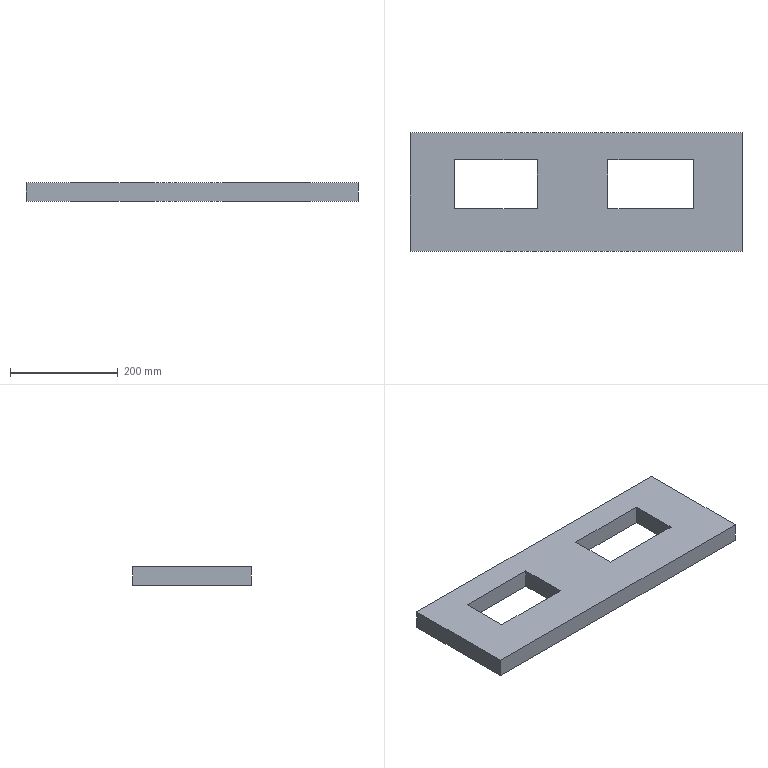Part | SolidWorks | features Extrusion 1, ICE 1 | 1 solid | 14 faces | box 616 x 220 x 35 mm | volume 3748166 mm3 | plane 14
STEP:
#1=CARTESIAN_POINT('',(308.,0.,17.5));
#2=VERTEX_POINT('',#1);
#3=CARTESIAN_POINT('',(308.,0.,-17.5));
#4=VERTEX_POINT('',#3);
#5=CARTESIAN_POINT('',(308.,0.,17.5));
#6=DIRECTION('',(0.,0.,-1.));
#7=VECTOR('',#6,1000.);
#8=LINE('',#5,#7);
#9=EDGE_CURVE('',#2,#4,#8,.T.);
#10=ORIENTED_EDGE('',*,*,#9,.T.);
#11=CARTESIAN_POINT('',(308.,220.,-17.5));
#12=VERTEX_POINT('',#11);
#13=CARTESIAN_POINT('',(308.,220.,-17.5));
#14=DIRECTION('',(0.,-1.,0.));
#15=VECTOR('',#14,1000.);
#16=LINE('',#13,#15);
#17=EDGE_CURVE('',#12,#4,#16,.T.);
#18=ORIENTED_EDGE('',*,*,#17,.F.);
#19=CARTESIAN_POINT('',(308.,220.,17.5));
#20=VERTEX_POINT('',#19);
#21=CARTESIAN_POINT('',(308.,220.,17.5));
#22=DIRECTION('',(0.,0.,-1.));
#23=VECTOR('',#22,1000.);
#24=LINE('',#21,#23);
#25=EDGE_CURVE('',#20,#12,#24,.T.);
#26=ORIENTED_EDGE('',*,*,#25,.F.);
#27=CARTESIAN_POINT('',(308.,220.,17.5));
#28=DIRECTION('',(0.,-1.,0.));
#29=VECTOR('',#28,1000.);
#30=LINE('',#27,#29);
#31=EDGE_CURVE('',#20,#2,#30,.T.);
#32=ORIENTED_EDGE('',*,*,#31,.T.);
#33=EDGE_LOOP('',(#10,#18,#26,#32));
#34=FACE_OUTER_BOUND('',#33,.T.);
#35=CARTESIAN_POINT('',(308.,220.,17.5));
#36=DIRECTION('',(-1.,0.,0.));
#37=DIRECTION('',(0.,0.,1.));
#38=AXIS2_PLACEMENT_3D('',#35,#36,#37);
#39=PLANE('',#38);
#40=ADVANCED_FACE('',(#34),#39,.F.);
#41=CARTESIAN_POINT('',(-225.575,79.078,-17.5));
#42=VERTEX_POINT('',#41);
#43=CARTESIAN_POINT('',(-71.632,79.078,-17.5));
#44=VERTEX_POINT('',#43);
#45=CARTESIAN_POINT('',(-225.575,79.078,-17.5));
#46=DIRECTION('',(1.,0.,0.));
#47=VECTOR('',#46,1000.);
#48=LINE('',#45,#47);
#49=EDGE_CURVE('',#42,#44,#48,.T.);
#50=ORIENTED_EDGE('',*,*,#49,.T.);
#51=CARTESIAN_POINT('',(-71.632,169.842,-17.5));
#52=VERTEX_POINT('',#51);
#53=CARTESIAN_POINT('',(-71.632,169.842,-17.5));
#54=DIRECTION('',(0.,1.,0.));
#55=VECTOR('',#54,1000.);
#56=LINE('',#53,#55);
#57=EDGE_CURVE('',#44,#52,#56,.T.);
#58=ORIENTED_EDGE('',*,*,#57,.T.);
#59=CARTESIAN_POINT('',(-225.575,169.842,-17.5));
#60=VERTEX_POINT('',#59);
#61=CARTESIAN_POINT('',(-225.575,169.842,-17.5));
#62=DIRECTION('',(-1.,0.,0.));
#63=VECTOR('',#62,1000.);
#64=LINE('',#61,#63);
#65=EDGE_CURVE('',#52,#60,#64,.T.);
#66=ORIENTED_EDGE('',*,*,#65,.T.);
#67=CARTESIAN_POINT('',(-225.575,169.842,-17.5));
#68=DIRECTION('',(0.,-1.,0.));
#69=VECTOR('',#68,1000.);
#70=LINE('',#67,#69);
#71=EDGE_CURVE('',#60,#42,#70,.T.);
#72=ORIENTED_EDGE('',*,*,#71,.T.);
#73=EDGE_LOOP('',(#50,#58,#66,#72));
#74=FACE_BOUND('',#73,.T.);
#75=CARTESIAN_POINT('',(59.175,79.078,-17.5));
#76=VERTEX_POINT('',#75);
#77=CARTESIAN_POINT('',(218.456,79.078,-17.5));
#78=VERTEX_POINT('',#77);
#79=CARTESIAN_POINT('',(59.175,79.078,-17.5));
#80=DIRECTION('',(1.,0.,0.));
#81=VECTOR('',#80,1000.);
#82=LINE('',#79,#81);
#83=EDGE_CURVE('',#76,#78,#82,.T.);
#84=ORIENTED_EDGE('',*,*,#83,.T.);
#85=CARTESIAN_POINT('',(218.456,169.842,-17.5));
#86=VERTEX_POINT('',#85);
#87=CARTESIAN_POINT('',(218.456,79.078,-17.5));
#88=DIRECTION('',(0.,1.,0.));
#89=VECTOR('',#88,1000.);
#90=LINE('',#87,#89);
#91=EDGE_CURVE('',#78,#86,#90,.T.);
#92=ORIENTED_EDGE('',*,*,#91,.T.);
#93=CARTESIAN_POINT('',(59.175,169.842,-17.5));
#94=VERTEX_POINT('',#93);
#95=CARTESIAN_POINT('',(59.175,169.842,-17.5));
#96=DIRECTION('',(-1.,0.,0.));
#97=VECTOR('',#96,1000.);
#98=LINE('',#95,#97);
#99=EDGE_CURVE('',#86,#94,#98,.T.);
#100=ORIENTED_EDGE('',*,*,#99,.T.);
#101=CARTESIAN_POINT('',(59.175,79.078,-17.5));
#102=DIRECTION('',(0.,-1.,0.));
#103=VECTOR('',#102,1000.);
#104=LINE('',#101,#103);
#105=EDGE_CURVE('',#94,#76,#104,.T.);
#106=ORIENTED_EDGE('',*,*,#105,.T.);
#107=EDGE_LOOP('',(#84,#92,#100,#106));
#108=FACE_BOUND('',#107,.T.);
#109=CARTESIAN_POINT('',(-308.,0.,-17.5));
#110=VERTEX_POINT('',#109);
#111=CARTESIAN_POINT('',(-308.,0.,-17.5));
#112=DIRECTION('',(-1.,0.,0.));
#113=VECTOR('',#112,1000.);
#114=LINE('',#111,#113);
#115=EDGE_CURVE('',#4,#110,#114,.T.);
#116=ORIENTED_EDGE('',*,*,#115,.T.);
#117=CARTESIAN_POINT('',(-308.,220.,-17.5));
#118=VERTEX_POINT('',#117);
#119=CARTESIAN_POINT('',(-308.,220.,-17.5));
#120=DIRECTION('',(0.,-1.,0.));
#121=VECTOR('',#120,1000.);
#122=LINE('',#119,#121);
#123=EDGE_CURVE('',#118,#110,#122,.T.);
#124=ORIENTED_EDGE('',*,*,#123,.F.);
#125=CARTESIAN_POINT('',(-308.,220.,-17.5));
#126=DIRECTION('',(-1.,0.,0.));
#127=VECTOR('',#126,1000.);
#128=LINE('',#125,#127);
#129=EDGE_CURVE('',#12,#118,#128,.T.);
#130=ORIENTED_EDGE('',*,*,#129,.F.);
#131=ORIENTED_EDGE('',*,*,#17,.T.);
#132=EDGE_LOOP('',(#116,#124,#130,#131));
#133=FACE_OUTER_BOUND('',#132,.T.);
#134=CARTESIAN_POINT('',(-308.,220.,-17.5));
#135=DIRECTION('',(0.,0.,1.));
#136=DIRECTION('',(1.,0.,0.));
#137=AXIS2_PLACEMENT_3D('',#134,#135,#136);
#138=PLANE('',#137);
#139=ADVANCED_FACE('',(#74,#108,#133),#138,.F.);
#140=CARTESIAN_POINT('',(-308.,0.,17.5));
#141=VERTEX_POINT('',#140);
#142=CARTESIAN_POINT('',(-308.,0.,17.5));
#143=DIRECTION('',(0.,0.,1.));
#144=VECTOR('',#143,1000.);
#145=LINE('',#142,#144);
#146=EDGE_CURVE('',#110,#141,#145,.T.);
#147=ORIENTED_EDGE('',*,*,#146,.T.);
#148=CARTESIAN_POINT('',(-308.,220.,17.5));
#149=VERTEX_POINT('',#148);
#150=CARTESIAN_POINT('',(-308.,220.,17.5));
#151=DIRECTION('',(0.,-1.,0.));
#152=VECTOR('',#151,1000.);
#153=LINE('',#150,#152);
#154=EDGE_CURVE('',#149,#141,#153,.T.);
#155=ORIENTED_EDGE('',*,*,#154,.F.);
#156=CARTESIAN_POINT('',(-308.,220.,17.5));
#157=DIRECTION('',(0.,0.,1.));
#158=VECTOR('',#157,1000.);
#159=LINE('',#156,#158);
#160=EDGE_CURVE('',#118,#149,#159,.T.);
#161=ORIENTED_EDGE('',*,*,#160,.F.);
#162=ORIENTED_EDGE('',*,*,#123,.T.);
#163=EDGE_LOOP('',(#147,#155,#161,#162));
#164=FACE_OUTER_BOUND('',#163,.T.);
#165=CARTESIAN_POINT('',(-308.,220.,17.5));
#166=DIRECTION('',(1.,0.,0.));
#167=DIRECTION('',(0.,0.,-1.));
#168=AXIS2_PLACEMENT_3D('',#165,#166,#167);
#169=PLANE('',#168);
#170=ADVANCED_FACE('',(#164),#169,.F.);
#171=CARTESIAN_POINT('',(-71.632,169.842,17.5));
#172=VERTEX_POINT('',#171);
#173=CARTESIAN_POINT('',(-225.575,169.842,17.5));
#174=VERTEX_POINT('',#173);
#175=CARTESIAN_POINT('',(-225.575,169.842,17.5));
#176=DIRECTION('',(-1.,0.,0.));
#177=VECTOR('',#176,1000.);
#178=LINE('',#175,#177);
#179=EDGE_CURVE('',#172,#174,#178,.T.);
#180=ORIENTED_EDGE('',*,*,#179,.F.);
#181=CARTESIAN_POINT('',(-71.632,79.078,17.5));
#182=VERTEX_POINT('',#181);
#183=CARTESIAN_POINT('',(-71.632,169.842,17.5));
#184=DIRECTION('',(0.,1.,0.));
#185=VECTOR('',#184,1000.);
#186=LINE('',#183,#185);
#187=EDGE_CURVE('',#182,#172,#186,.T.);
#188=ORIENTED_EDGE('',*,*,#187,.F.);
#189=CARTESIAN_POINT('',(-225.575,79.078,17.5));
#190=VERTEX_POINT('',#189);
#191=CARTESIAN_POINT('',(-225.575,79.078,17.5));
#192=DIRECTION('',(1.,0.,0.));
#193=VECTOR('',#192,1000.);
#194=LINE('',#191,#193);
#195=EDGE_CURVE('',#190,#182,#194,.T.);
#196=ORIENTED_EDGE('',*,*,#195,.F.);
#197=CARTESIAN_POINT('',(-225.575,169.842,17.5));
#198=DIRECTION('',(0.,-1.,0.));
#199=VECTOR('',#198,1000.);
#200=LINE('',#197,#199);
#201=EDGE_CURVE('',#174,#190,#200,.T.);
#202=ORIENTED_EDGE('',*,*,#201,.F.);
#203=EDGE_LOOP('',(#180,#188,#196,#202));
#204=FACE_BOUND('',#203,.T.);
#205=CARTESIAN_POINT('',(218.456,169.842,17.5));
#206=VERTEX_POINT('',#205);
#207=CARTESIAN_POINT('',(59.175,169.842,17.5));
#208=VERTEX_POINT('',#207);
#209=CARTESIAN_POINT('',(59.175,169.842,17.5));
#210=DIRECTION('',(-1.,0.,0.));
#211=VECTOR('',#210,1000.);
#212=LINE('',#209,#211);
#213=EDGE_CURVE('',#206,#208,#212,.T.);
#214=ORIENTED_EDGE('',*,*,#213,.F.);
#215=CARTESIAN_POINT('',(218.456,79.078,17.5));
#216=VERTEX_POINT('',#215);
#217=CARTESIAN_POINT('',(218.456,79.078,17.5));
#218=DIRECTION('',(0.,1.,0.));
#219=VECTOR('',#218,1000.);
#220=LINE('',#217,#219);
#221=EDGE_CURVE('',#216,#206,#220,.T.);
#222=ORIENTED_EDGE('',*,*,#221,.F.);
#223=CARTESIAN_POINT('',(59.175,79.078,17.5));
#224=VERTEX_POINT('',#223);
#225=CARTESIAN_POINT('',(59.175,79.078,17.5));
#226=DIRECTION('',(1.,0.,0.));
#227=VECTOR('',#226,1000.);
#228=LINE('',#225,#227);
#229=EDGE_CURVE('',#224,#216,#228,.T.);
#230=ORIENTED_EDGE('',*,*,#229,.F.);
#231=CARTESIAN_POINT('',(59.175,79.078,17.5));
#232=DIRECTION('',(0.,-1.,0.));
#233=VECTOR('',#232,1000.);
#234=LINE('',#231,#233);
#235=EDGE_CURVE('',#208,#224,#234,.T.);
#236=ORIENTED_EDGE('',*,*,#235,.F.);
#237=EDGE_LOOP('',(#214,#222,#230,#236));
#238=FACE_BOUND('',#237,.T.);
#239=CARTESIAN_POINT('',(-308.,0.,17.5));
#240=DIRECTION('',(1.,0.,0.));
#241=VECTOR('',#240,1000.);
#242=LINE('',#239,#241);
#243=EDGE_CURVE('',#141,#2,#242,.T.);
#244=ORIENTED_EDGE('',*,*,#243,.T.);
#245=ORIENTED_EDGE('',*,*,#31,.F.);
#246=CARTESIAN_POINT('',(-308.,220.,17.5));
#247=DIRECTION('',(1.,0.,0.));
#248=VECTOR('',#247,1000.);
#249=LINE('',#246,#248);
#250=EDGE_CURVE('',#149,#20,#249,.T.);
#251=ORIENTED_EDGE('',*,*,#250,.F.);
#252=ORIENTED_EDGE('',*,*,#154,.T.);
#253=EDGE_LOOP('',(#244,#245,#251,#252));
#254=FACE_OUTER_BOUND('',#253,.T.);
#255=CARTESIAN_POINT('',(-308.,220.,17.5));
#256=DIRECTION('',(0.,0.,-1.));
#257=DIRECTION('',(-1.,0.,0.));
#258=AXIS2_PLACEMENT_3D('',#255,#256,#257);
#259=PLANE('',#258);
#260=ADVANCED_FACE('',(#204,#238,#254),#259,.F.);
#261=ORIENTED_EDGE('',*,*,#25,.T.);
#262=ORIENTED_EDGE('',*,*,#129,.T.);
#263=ORIENTED_EDGE('',*,*,#160,.T.);
#264=ORIENTED_EDGE('',*,*,#250,.T.);
#265=EDGE_LOOP('',(#261,#262,#263,#264));
#266=FACE_OUTER_BOUND('',#265,.T.);
#267=CARTESIAN_POINT('',(0.,220.,0.));
#268=DIRECTION('',(0.,-1.,0.));
#269=DIRECTION('',(0.,0.,-1.));
#270=AXIS2_PLACEMENT_3D('',#267,#268,#269);
#271=PLANE('',#270);
#272=ADVANCED_FACE('',(#266),#271,.F.);
#273=ORIENTED_EDGE('',*,*,#9,.F.);
#274=ORIENTED_EDGE('',*,*,#243,.F.);
#275=ORIENTED_EDGE('',*,*,#146,.F.);
#276=ORIENTED_EDGE('',*,*,#115,.F.);
#277=EDGE_LOOP('',(#273,#274,#275,#276));
#278=FACE_OUTER_BOUND('',#277,.T.);
#279=CARTESIAN_POINT('',(0.,0.,0.));
#280=DIRECTION('',(0.,-1.,0.));
#281=DIRECTION('',(0.,0.,-1.));
#282=AXIS2_PLACEMENT_3D('',#279,#280,#281);
#283=PLANE('',#282);
#284=ADVANCED_FACE('',(#278),#283,.T.);
#285=ORIENTED_EDGE('',*,*,#221,.T.);
#286=CARTESIAN_POINT('',(218.456,169.842,-17.5));
#287=DIRECTION('',(0.,0.,1.));
#288=VECTOR('',#287,1000.);
#289=LINE('',#286,#288);
#290=EDGE_CURVE('',#86,#206,#289,.T.);
#291=ORIENTED_EDGE('',*,*,#290,.F.);
#292=ORIENTED_EDGE('',*,*,#91,.F.);
#293=CARTESIAN_POINT('',(218.456,79.078,-17.5));
#294=DIRECTION('',(0.,0.,1.));
#295=VECTOR('',#294,1000.);
#296=LINE('',#293,#295);
#297=EDGE_CURVE('',#78,#216,#296,.T.);
#298=ORIENTED_EDGE('',*,*,#297,.T.);
#299=EDGE_LOOP('',(#285,#291,#292,#298));
#300=FACE_OUTER_BOUND('',#299,.T.);
#301=CARTESIAN_POINT('',(218.456,79.078,-17.5));
#302=DIRECTION('',(1.,0.,0.));
#303=DIRECTION('',(0.,0.,-1.));
#304=AXIS2_PLACEMENT_3D('',#301,#302,#303);
#305=PLANE('',#304);
#306=ADVANCED_FACE('',(#300),#305,.F.);
#307=ORIENTED_EDGE('',*,*,#229,.T.);
#308=ORIENTED_EDGE('',*,*,#297,.F.);
#309=ORIENTED_EDGE('',*,*,#83,.F.);
#310=CARTESIAN_POINT('',(59.175,79.078,-17.5));
#311=DIRECTION('',(0.,0.,1.));
#312=VECTOR('',#311,1000.);
#313=LINE('',#310,#312);
#314=EDGE_CURVE('',#76,#224,#313,.T.);
#315=ORIENTED_EDGE('',*,*,#314,.T.);
#316=EDGE_LOOP('',(#307,#308,#309,#315));
#317=FACE_OUTER_BOUND('',#316,.T.);
#318=CARTESIAN_POINT('',(59.175,79.078,-17.5));
#319=DIRECTION('',(0.,-1.,0.));
#320=DIRECTION('',(0.,0.,-1.));
#321=AXIS2_PLACEMENT_3D('',#318,#319,#320);
#322=PLANE('',#321);
#323=ADVANCED_FACE('',(#317),#322,.F.);
#324=ORIENTED_EDGE('',*,*,#235,.T.);
#325=ORIENTED_EDGE('',*,*,#314,.F.);
#326=ORIENTED_EDGE('',*,*,#105,.F.);
#327=CARTESIAN_POINT('',(59.175,169.842,-17.5));
#328=DIRECTION('',(0.,0.,1.));
#329=VECTOR('',#328,1000.);
#330=LINE('',#327,#329);
#331=EDGE_CURVE('',#94,#208,#330,.T.);
#332=ORIENTED_EDGE('',*,*,#331,.T.);
#333=EDGE_LOOP('',(#324,#325,#326,#332));
#334=FACE_OUTER_BOUND('',#333,.T.);
#335=CARTESIAN_POINT('',(59.175,79.078,-17.5));
#336=DIRECTION('',(-1.,0.,0.));
#337=DIRECTION('',(0.,0.,1.));
#338=AXIS2_PLACEMENT_3D('',#335,#336,#337);
#339=PLANE('',#338);
#340=ADVANCED_FACE('',(#334),#339,.F.);
#341=ORIENTED_EDGE('',*,*,#213,.T.);
#342=ORIENTED_EDGE('',*,*,#331,.F.);
#343=ORIENTED_EDGE('',*,*,#99,.F.);
#344=ORIENTED_EDGE('',*,*,#290,.T.);
#345=EDGE_LOOP('',(#341,#342,#343,#344));
#346=FACE_OUTER_BOUND('',#345,.T.);
#347=CARTESIAN_POINT('',(59.175,169.842,-17.5));
#348=DIRECTION('',(0.,1.,0.));
#349=DIRECTION('',(0.,0.,1.));
#350=AXIS2_PLACEMENT_3D('',#347,#348,#349);
#351=PLANE('',#350);
#352=ADVANCED_FACE('',(#346),#351,.F.);
#353=ORIENTED_EDGE('',*,*,#187,.T.);
#354=CARTESIAN_POINT('',(-71.632,169.842,-17.5));
#355=DIRECTION('',(0.,0.,1.));
#356=VECTOR('',#355,1000.);
#357=LINE('',#354,#356);
#358=EDGE_CURVE('',#52,#172,#357,.T.);
#359=ORIENTED_EDGE('',*,*,#358,.F.);
#360=ORIENTED_EDGE('',*,*,#57,.F.);
#361=CARTESIAN_POINT('',(-71.632,79.078,-17.5));
#362=DIRECTION('',(0.,0.,1.));
#363=VECTOR('',#362,1000.);
#364=LINE('',#361,#363);
#365=EDGE_CURVE('',#44,#182,#364,.T.);
#366=ORIENTED_EDGE('',*,*,#365,.T.);
#367=EDGE_LOOP('',(#353,#359,#360,#366));
#368=FACE_OUTER_BOUND('',#367,.T.);
#369=CARTESIAN_POINT('',(-71.632,169.842,-17.5));
#370=DIRECTION('',(1.,0.,0.));
#371=DIRECTION('',(0.,0.,-1.));
#372=AXIS2_PLACEMENT_3D('',#369,#370,#371);
#373=PLANE('',#372);
#374=ADVANCED_FACE('',(#368),#373,.F.);
#375=ORIENTED_EDGE('',*,*,#195,.T.);
#376=ORIENTED_EDGE('',*,*,#365,.F.);
#377=ORIENTED_EDGE('',*,*,#49,.F.);
#378=CARTESIAN_POINT('',(-225.575,79.078,-17.5));
#379=DIRECTION('',(0.,0.,1.));
#380=VECTOR('',#379,1000.);
#381=LINE('',#378,#380);
#382=EDGE_CURVE('',#42,#190,#381,.T.);
#383=ORIENTED_EDGE('',*,*,#382,.T.);
#384=EDGE_LOOP('',(#375,#376,#377,#383));
#385=FACE_OUTER_BOUND('',#384,.T.);
#386=CARTESIAN_POINT('',(-225.575,79.078,-17.5));
#387=DIRECTION('',(0.,-1.,0.));
#388=DIRECTION('',(0.,0.,-1.));
#389=AXIS2_PLACEMENT_3D('',#386,#387,#388);
#390=PLANE('',#389);
#391=ADVANCED_FACE('',(#385),#390,.F.);
#392=ORIENTED_EDGE('',*,*,#201,.T.);
#393=ORIENTED_EDGE('',*,*,#382,.F.);
#394=ORIENTED_EDGE('',*,*,#71,.F.);
#395=CARTESIAN_POINT('',(-225.575,169.842,-17.5));
#396=DIRECTION('',(0.,0.,1.));
#397=VECTOR('',#396,1000.);
#398=LINE('',#395,#397);
#399=EDGE_CURVE('',#60,#174,#398,.T.);
#400=ORIENTED_EDGE('',*,*,#399,.T.);
#401=EDGE_LOOP('',(#392,#393,#394,#400));
#402=FACE_OUTER_BOUND('',#401,.T.);
#403=CARTESIAN_POINT('',(-225.575,169.842,-17.5));
#404=DIRECTION('',(-1.,0.,0.));
#405=DIRECTION('',(0.,0.,1.));
#406=AXIS2_PLACEMENT_3D('',#403,#404,#405);
#407=PLANE('',#406);
#408=ADVANCED_FACE('',(#402),#407,.F.);
#409=ORIENTED_EDGE('',*,*,#179,.T.);
#410=ORIENTED_EDGE('',*,*,#399,.F.);
#411=ORIENTED_EDGE('',*,*,#65,.F.);
#412=ORIENTED_EDGE('',*,*,#358,.T.);
#413=EDGE_LOOP('',(#409,#410,#411,#412));
#414=FACE_OUTER_BOUND('',#413,.T.);
#415=CARTESIAN_POINT('',(-225.575,169.842,-17.5));
#416=DIRECTION('',(0.,1.,0.));
#417=DIRECTION('',(0.,0.,1.));
#418=AXIS2_PLACEMENT_3D('',#415,#416,#417);
#419=PLANE('',#418);
#420=ADVANCED_FACE('',(#414),#419,.F.);
#421=CLOSED_SHELL('',(#40,#139,#170,#260,#272,#284,#306,#323,#340,#352,#374,#391,#408,#420));
#422=MANIFOLD_SOLID_BREP('',#421);
#423=CARTESIAN_POINT('',(0.,0.,0.));
#424=DIRECTION('',(0.,0.,1.));
#425=DIRECTION('',(1.,0.,0.));
#426=AXIS2_PLACEMENT_3D('',#423,#424,#425);
#427=(LENGTH_UNIT()NAMED_UNIT(*)SI_UNIT(.MILLI.,.METRE.));
#428=UNCERTAINTY_MEASURE_WITH_UNIT(LENGTH_MEASURE(0.00001),#427,'','');
#429=(NAMED_UNIT(*)PLANE_ANGLE_UNIT()SI_UNIT($,.RADIAN.));
#430=(NAMED_UNIT(*)SI_UNIT($,.STERADIAN.)SOLID_ANGLE_UNIT());
#431=(GEOMETRIC_REPRESENTATION_CONTEXT(3)GLOBAL_UNCERTAINTY_ASSIGNED_CONTEXT((#428))GLOBAL_UNIT_ASSIGNED_CONTEXT((#427,#429,#430))REPRESENTATION_CONTEXT('',''));
#432=ADVANCED_BREP_SHAPE_REPRESENTATION('',(#422,#426),#431);